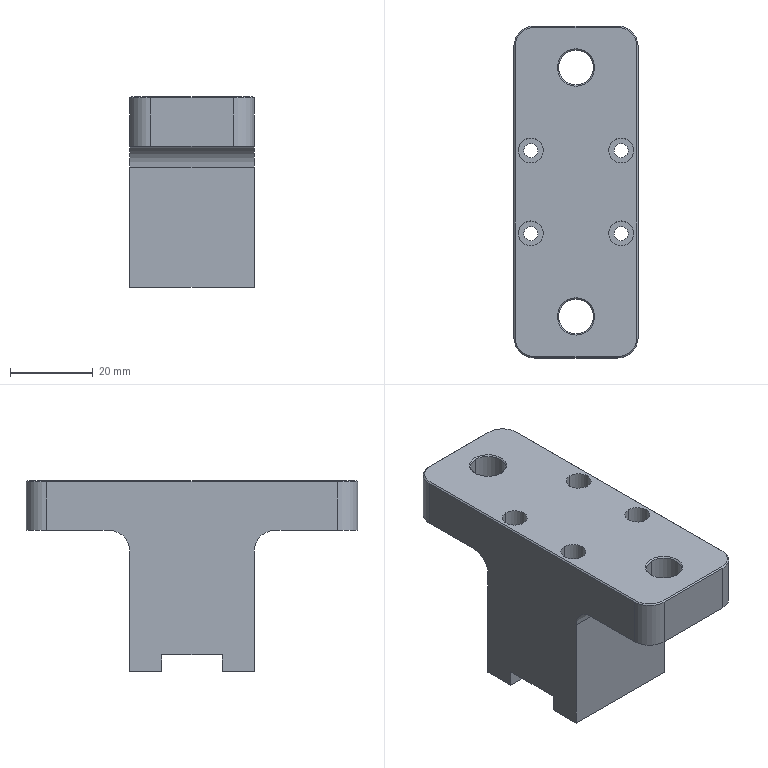Part | 1 solid | 60 faces | box 30 x 80 x 46 mm | volume 52099 mm3 | cylinder 26 | plane 22 | cone 12 | commonest cylinder face diameters 3.4 x8 6 x8 10 x6 8.4 x4